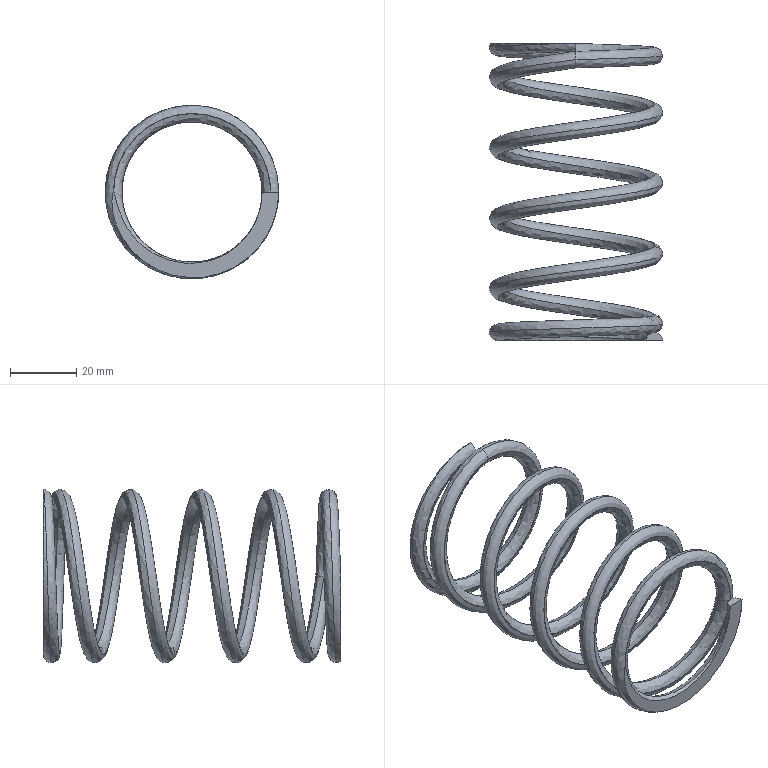Part | SolidWorks | features Sweep 3, ICE 1 | 1 solid | 22 faces | box 52.5 x 90 x 52.5 mm | volume 16226 mm3 | spline 18 | plane 4